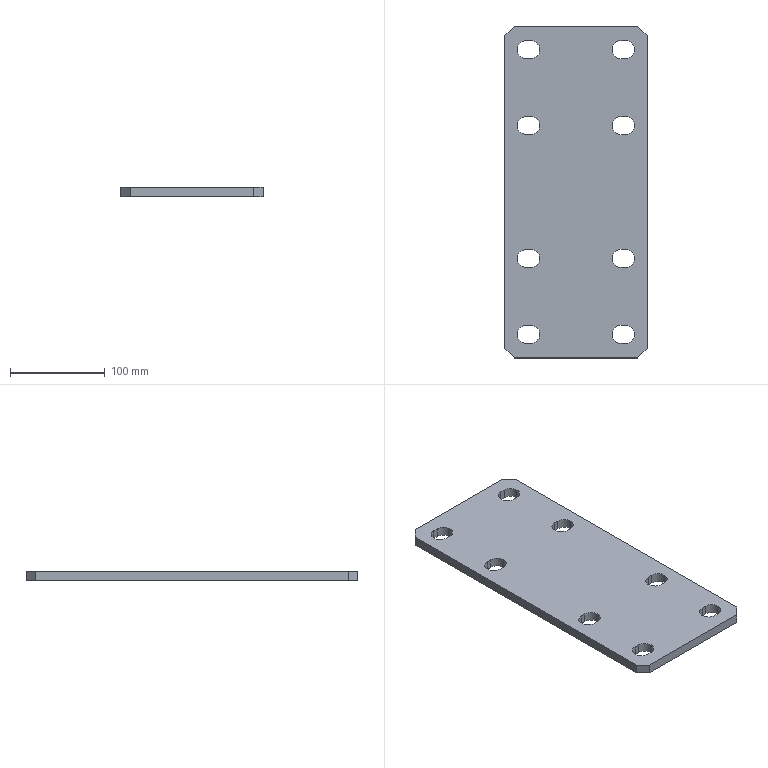Part | STEP file | E3-立柱外敷Plate | 1 solid | 50 faces | box 150 x 350 x 10 mm | volume 492718 mm3 | plane 26 | cylinder 24 | commonest cylinder face diameters 19 x24